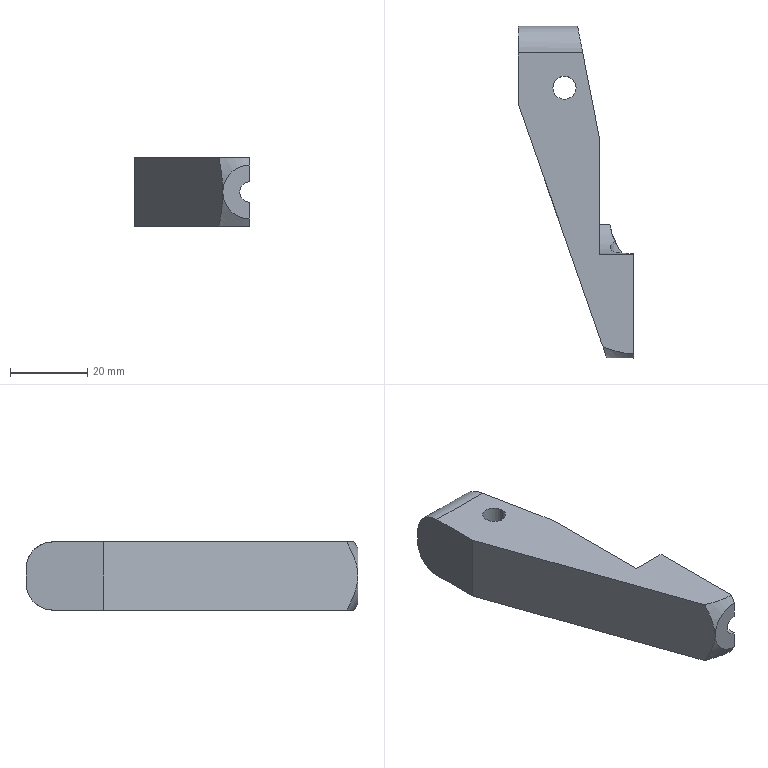Part | SolidWorks | features ICE 6, Extrusion 1, Fillet 1, RevCut 1 | 1 solid | 25 faces | box 30 x 86 x 17.7 mm | volume 18921 mm3 | plane 11 | cylinder 8 | spline 2 | torus 2 | cone 2 | commonest cylinder face diameters 6 x2 8 x2 14 x2 5.3 x1 12.388 x1
STEP:
#1=CARTESIAN_POINT('',(16.36,-5.,4.85));
#2=VERTEX_POINT('',#1);
#3=CARTESIAN_POINT('',(16.36,-5.,12.85));
#4=VERTEX_POINT('',#3);
#5=CARTESIAN_POINT('',(16.36,-5.,4.85));
#6=CARTESIAN_POINT('',(17.933,-13.,4.85));
#7=CARTESIAN_POINT('',(17.933,-13.,12.85));
#8=CARTESIAN_POINT('',(16.36,-5.,12.85));
#9=(BOUNDED_CURVE()B_SPLINE_CURVE(3,(#5,#6,#7,#8),.UNSPECIFIED.,.F.,.F.)B_SPLINE_CURVE_WITH_KNOTS((4,4),(1.571,4.712),.UNSPECIFIED.)CURVE()GEOMETRIC_REPRESENTATION_ITEM()RATIONAL_B_SPLINE_CURVE((1.,0.3333,0.3333,1.))REPRESENTATION_ITEM(''));
#10=EDGE_CURVE('',#2,#4,#9,.T.);
#11=ORIENTED_EDGE('',*,*,#10,.F.);
#12=CARTESIAN_POINT('',(6.,-5.,4.85));
#13=VERTEX_POINT('',#12);
#14=CARTESIAN_POINT('',(54.,-5.,4.85));
#15=DIRECTION('',(-1.,0.,0.));
#16=VECTOR('',#15,1000.);
#17=LINE('',#14,#16);
#18=EDGE_CURVE('',#2,#13,#17,.T.);
#19=ORIENTED_EDGE('',*,*,#18,.T.);
#20=CARTESIAN_POINT('',(6.,-5.,12.85));
#21=VERTEX_POINT('',#20);
#22=CARTESIAN_POINT('',(6.,-5.,8.85));
#23=DIRECTION('',(-1.,0.,0.));
#24=DIRECTION('',(0.,0.,1.));
#25=AXIS2_PLACEMENT_3D('',#22,#23,#24);
#26=CIRCLE('',#25,4.);
#27=EDGE_CURVE('',#13,#21,#26,.T.);
#28=ORIENTED_EDGE('',*,*,#27,.T.);
#29=CARTESIAN_POINT('',(54.,-5.,12.85));
#30=DIRECTION('',(-1.,0.,0.));
#31=VECTOR('',#30,1000.);
#32=LINE('',#29,#31);
#33=EDGE_CURVE('',#4,#21,#32,.T.);
#34=ORIENTED_EDGE('',*,*,#33,.F.);
#35=EDGE_LOOP('',(#11,#19,#28,#34));
#36=FACE_OUTER_BOUND('',#35,.T.);
#37=CARTESIAN_POINT('',(54.,-5.,8.85));
#38=DIRECTION('',(-1.,0.,0.));
#39=DIRECTION('',(0.,0.,1.));
#40=AXIS2_PLACEMENT_3D('',#37,#38,#39);
#41=CYLINDRICAL_SURFACE('',#40,4.);
#42=ADVANCED_FACE('',(#36),#41,.F.);
#43=CARTESIAN_POINT('',(9.,-16.,17.7));
#44=VERTEX_POINT('',#43);
#45=CARTESIAN_POINT('',(15.,-16.,17.7));
#46=VERTEX_POINT('',#45);
#47=CARTESIAN_POINT('',(12.,-16.,17.7));
#48=DIRECTION('',(0.,0.,1.));
#49=DIRECTION('',(1.,0.,0.));
#50=AXIS2_PLACEMENT_3D('',#47,#48,#49);
#51=CIRCLE('',#50,3.);
#52=EDGE_CURVE('',#44,#46,#51,.T.);
#53=ORIENTED_EDGE('',*,*,#52,.T.);
#54=CARTESIAN_POINT('',(15.,-16.,0.));
#55=VERTEX_POINT('',#54);
#56=CARTESIAN_POINT('',(15.,-16.,17.7));
#57=DIRECTION('',(0.,0.,-1.));
#58=VECTOR('',#57,1000.);
#59=LINE('',#56,#58);
#60=EDGE_CURVE('',#46,#55,#59,.T.);
#61=ORIENTED_EDGE('',*,*,#60,.T.);
#62=CARTESIAN_POINT('',(9.,-16.,0.));
#63=VERTEX_POINT('',#62);
#64=CARTESIAN_POINT('',(12.,-16.,0.));
#65=DIRECTION('',(0.,0.,1.));
#66=DIRECTION('',(1.,0.,0.));
#67=AXIS2_PLACEMENT_3D('',#64,#65,#66);
#68=CIRCLE('',#67,3.);
#69=EDGE_CURVE('',#63,#55,#68,.T.);
#70=ORIENTED_EDGE('',*,*,#69,.F.);
#71=CARTESIAN_POINT('',(9.,-16.,17.7));
#72=DIRECTION('',(0.,0.,-1.));
#73=VECTOR('',#72,1000.);
#74=LINE('',#71,#73);
#75=EDGE_CURVE('',#44,#63,#74,.T.);
#76=ORIENTED_EDGE('',*,*,#75,.F.);
#77=EDGE_LOOP('',(#53,#61,#70,#76));
#78=FACE_OUTER_BOUND('',#77,.T.);
#79=CARTESIAN_POINT('',(12.,-16.,17.7));
#80=DIRECTION('',(0.,0.,-1.));
#81=DIRECTION('',(-1.,0.,0.));
#82=AXIS2_PLACEMENT_3D('',#79,#80,#81);
#83=CYLINDRICAL_SURFACE('',#82,3.);
#84=ADVANCED_FACE('',(#78),#83,.F.);
#85=CARTESIAN_POINT('',(30.,-59.152,17.7));
#86=VERTEX_POINT('',#85);
#87=CARTESIAN_POINT('',(30.,-84.932,17.7));
#88=VERTEX_POINT('',#87);
#89=CARTESIAN_POINT('',(30.,-86.,17.7));
#90=DIRECTION('',(0.,-1.,0.));
#91=VECTOR('',#90,1000.);
#92=LINE('',#89,#91);
#93=EDGE_CURVE('',#86,#88,#92,.T.);
#94=ORIENTED_EDGE('',*,*,#93,.F.);
#95=CARTESIAN_POINT('',(21.,-59.152,17.7));
#96=VERTEX_POINT('',#95);
#97=CARTESIAN_POINT('',(58.282,-59.152,17.7));
#98=DIRECTION('',(-1.,0.,0.));
#99=VECTOR('',#98,1000.);
#100=LINE('',#97,#99);
#101=EDGE_CURVE('',#86,#96,#100,.T.);
#102=ORIENTED_EDGE('',*,*,#101,.T.);
#103=CARTESIAN_POINT('',(21.,-28.6,17.7));
#104=VERTEX_POINT('',#103);
#105=CARTESIAN_POINT('',(21.,-51.504,17.7));
#106=DIRECTION('',(0.,1.,0.));
#107=VECTOR('',#106,1000.);
#108=LINE('',#105,#107);
#109=EDGE_CURVE('',#96,#104,#108,.T.);
#110=ORIENTED_EDGE('',*,*,#109,.T.);
#111=CARTESIAN_POINT('',(16.753,-7.,17.7));
#112=VERTEX_POINT('',#111);
#113=CARTESIAN_POINT('',(21.,-28.6,17.7));
#114=DIRECTION('',(-0.1929,0.9812,0.));
#115=VECTOR('',#114,1000.);
#116=LINE('',#113,#115);
#117=EDGE_CURVE('',#104,#112,#116,.T.);
#118=ORIENTED_EDGE('',*,*,#117,.T.);
#119=CARTESIAN_POINT('',(0.,-7.,17.7));
#120=VERTEX_POINT('',#119);
#121=CARTESIAN_POINT('',(0.,-7.,17.7));
#122=DIRECTION('',(-1.,0.,0.));
#123=VECTOR('',#122,1000.);
#124=LINE('',#121,#123);
#125=EDGE_CURVE('',#112,#120,#124,.T.);
#126=ORIENTED_EDGE('',*,*,#125,.T.);
#127=CARTESIAN_POINT('',(0.,-20.136,17.7));
#128=VERTEX_POINT('',#127);
#129=CARTESIAN_POINT('',(0.,-20.136,17.7));
#130=DIRECTION('',(0.,-1.,0.));
#131=VECTOR('',#130,1000.);
#132=LINE('',#129,#131);
#133=EDGE_CURVE('',#120,#128,#132,.T.);
#134=ORIENTED_EDGE('',*,*,#133,.T.);
#135=CARTESIAN_POINT('',(21.049,-80.412,17.7));
#136=VERTEX_POINT('',#135);
#137=CARTESIAN_POINT('',(21.049,-80.412,17.7));
#138=DIRECTION('',(0.3297,-0.9441,0.));
#139=VECTOR('',#138,1000.);
#140=LINE('',#137,#139);
#141=EDGE_CURVE('',#128,#136,#140,.T.);
#142=ORIENTED_EDGE('',*,*,#141,.T.);
#143=CARTESIAN_POINT('',(21.669,-82.189,17.7));
#144=VERTEX_POINT('',#143);
#145=CARTESIAN_POINT('',(21.049,-80.412,17.7));
#146=CARTESIAN_POINT('',(21.259,-81.015,17.7));
#147=CARTESIAN_POINT('',(21.467,-81.609,17.7));
#148=CARTESIAN_POINT('',(21.669,-82.189,17.7));
#149=B_SPLINE_CURVE_WITH_KNOTS('',3,(#145,#146,#147,#148),.UNSPECIFIED.,.F.,.F.,(4,4),(0.75,1.),.UNSPECIFIED.);
#150=EDGE_CURVE('',#136,#144,#149,.T.);
#151=ORIENTED_EDGE('',*,*,#150,.T.);
#152=CARTESIAN_POINT('',(22.007,-83.156,17.7));
#153=VERTEX_POINT('',#152);
#154=CARTESIAN_POINT('',(21.669,-82.189,17.7));
#155=CARTESIAN_POINT('',(21.784,-82.517,17.7));
#156=CARTESIAN_POINT('',(21.897,-82.841,17.7));
#157=CARTESIAN_POINT('',(22.007,-83.156,17.7));
#158=B_SPLINE_CURVE_WITH_KNOTS('',3,(#154,#155,#156,#157),.UNSPECIFIED.,.F.,.F.,(4,4),(0.5,0.6415),.UNSPECIFIED.);
#159=EDGE_CURVE('',#144,#153,#158,.T.);
#160=ORIENTED_EDGE('',*,*,#159,.T.);
#161=CARTESIAN_POINT('',(22.007,-83.156,17.7));
#162=CARTESIAN_POINT('',(23.287,-83.652,17.7));
#163=CARTESIAN_POINT('',(24.588,-84.094,17.7));
#164=CARTESIAN_POINT('',(26.602,-84.58,17.7));
#165=CARTESIAN_POINT('',(27.28,-84.71,17.7));
#166=CARTESIAN_POINT('',(28.637,-84.886,17.7));
#167=CARTESIAN_POINT('',(29.317,-84.932,17.7));
#168=CARTESIAN_POINT('',(30.,-84.932,17.7));
#169=B_SPLINE_CURVE_WITH_KNOTS('',3,(#161,#162,#163,#164,#165,#166,#167,#168),.UNSPECIFIED.,.F.,.F.,(4,2,2,4),(0.1132,0.1173,0.1194,0.1214),.UNSPECIFIED.);
#170=EDGE_CURVE('',#153,#88,#169,.T.);
#171=ORIENTED_EDGE('',*,*,#170,.T.);
#172=EDGE_LOOP('',(#94,#102,#110,#118,#126,#134,#142,#151,#160,#171));
#173=FACE_OUTER_BOUND('',#172,.T.);
#174=ORIENTED_EDGE('',*,*,#52,.F.);
#175=CARTESIAN_POINT('',(12.,-16.,17.7));
#176=DIRECTION('',(0.,0.,1.));
#177=DIRECTION('',(1.,0.,0.));
#178=AXIS2_PLACEMENT_3D('',#175,#176,#177);
#179=CIRCLE('',#178,3.);
#180=EDGE_CURVE('',#46,#44,#179,.T.);
#181=ORIENTED_EDGE('',*,*,#180,.F.);
#182=EDGE_LOOP('',(#174,#181));
#183=FACE_BOUND('',#182,.T.);
#184=CARTESIAN_POINT('',(25.162,-51.504,17.7));
#185=DIRECTION('',(0.,0.,1.));
#186=DIRECTION('',(1.,0.,0.));
#187=AXIS2_PLACEMENT_3D('',#184,#185,#186);
#188=PLANE('',#187);
#189=ADVANCED_FACE('',(#173,#183),#188,.T.);
#190=ORIENTED_EDGE('',*,*,#69,.T.);
#191=CARTESIAN_POINT('',(12.,-16.,0.));
#192=DIRECTION('',(0.,0.,1.));
#193=DIRECTION('',(1.,0.,0.));
#194=AXIS2_PLACEMENT_3D('',#191,#192,#193);
#195=CIRCLE('',#194,3.);
#196=EDGE_CURVE('',#55,#63,#195,.T.);
#197=ORIENTED_EDGE('',*,*,#196,.T.);
#198=EDGE_LOOP('',(#190,#197));
#199=FACE_BOUND('',#198,.T.);
#200=CARTESIAN_POINT('',(30.,-60.226,0.));
#201=VERTEX_POINT('',#200);
#202=CARTESIAN_POINT('',(23.784,-51.504,0.));
#203=VERTEX_POINT('',#202);
#204=CARTESIAN_POINT('',(30.,-60.226,0.));
#205=CARTESIAN_POINT('',(27.027,-60.226,0.));
#206=CARTESIAN_POINT('',(24.641,-56.878,0.));
#207=CARTESIAN_POINT('',(23.784,-51.504,0.));
#208=(BOUNDED_CURVE()B_SPLINE_CURVE(3,(#204,#205,#206,#207),.UNSPECIFIED.,.F.,.F.)B_SPLINE_CURVE_WITH_KNOTS((4,4),(3.142,4.42),.UNSPECIFIED.)CURVE()GEOMETRIC_REPRESENTATION_ITEM()RATIONAL_B_SPLINE_CURVE((1.,0.8684,0.8684,1.))REPRESENTATION_ITEM(''));
#209=EDGE_CURVE('',#201,#203,#208,.T.);
#210=ORIENTED_EDGE('',*,*,#209,.F.);
#211=CARTESIAN_POINT('',(30.,-84.932,0.));
#212=VERTEX_POINT('',#211);
#213=CARTESIAN_POINT('',(30.,-51.504,0.));
#214=DIRECTION('',(0.,-1.,0.));
#215=VECTOR('',#214,1000.);
#216=LINE('',#213,#215);
#217=EDGE_CURVE('',#201,#212,#216,.T.);
#218=ORIENTED_EDGE('',*,*,#217,.T.);
#219=CARTESIAN_POINT('',(22.007,-83.156,0.));
#220=VERTEX_POINT('',#219);
#221=CARTESIAN_POINT('',(22.007,-83.156,0.));
#222=CARTESIAN_POINT('',(23.287,-83.652,0.));
#223=CARTESIAN_POINT('',(24.588,-84.094,0.));
#224=CARTESIAN_POINT('',(26.602,-84.58,0.));
#225=CARTESIAN_POINT('',(27.28,-84.71,0.));
#226=CARTESIAN_POINT('',(28.637,-84.886,0.));
#227=CARTESIAN_POINT('',(29.317,-84.932,0.));
#228=CARTESIAN_POINT('',(30.,-84.932,0.));
#229=B_SPLINE_CURVE_WITH_KNOTS('',3,(#221,#222,#223,#224,#225,#226,#227,#228),.UNSPECIFIED.,.F.,.F.,(4,2,2,4),(0.1132,0.1173,0.1194,0.1214),.UNSPECIFIED.);
#230=EDGE_CURVE('',#220,#212,#229,.T.);
#231=ORIENTED_EDGE('',*,*,#230,.F.);
#232=CARTESIAN_POINT('',(21.669,-82.189,0.));
#233=VERTEX_POINT('',#232);
#234=CARTESIAN_POINT('',(21.669,-82.189,0.));
#235=CARTESIAN_POINT('',(21.784,-82.517,0.));
#236=CARTESIAN_POINT('',(21.897,-82.841,0.));
#237=CARTESIAN_POINT('',(22.007,-83.156,0.));
#238=B_SPLINE_CURVE_WITH_KNOTS('',3,(#234,#235,#236,#237),.UNSPECIFIED.,.F.,.F.,(4,4),(0.5,0.6415),.UNSPECIFIED.);
#239=EDGE_CURVE('',#233,#220,#238,.T.);
#240=ORIENTED_EDGE('',*,*,#239,.F.);
#241=CARTESIAN_POINT('',(21.049,-80.412,0.));
#242=VERTEX_POINT('',#241);
#243=CARTESIAN_POINT('',(21.049,-80.412,0.));
#244=CARTESIAN_POINT('',(21.259,-81.015,0.));
#245=CARTESIAN_POINT('',(21.467,-81.609,0.));
#246=CARTESIAN_POINT('',(21.669,-82.189,0.));
#247=B_SPLINE_CURVE_WITH_KNOTS('',3,(#243,#244,#245,#246),.UNSPECIFIED.,.F.,.F.,(4,4),(0.75,1.),.UNSPECIFIED.);
#248=EDGE_CURVE('',#242,#233,#247,.T.);
#249=ORIENTED_EDGE('',*,*,#248,.F.);
#250=CARTESIAN_POINT('',(0.,-20.136,0.));
#251=VERTEX_POINT('',#250);
#252=CARTESIAN_POINT('',(21.049,-80.412,0.));
#253=DIRECTION('',(0.3297,-0.9441,0.));
#254=VECTOR('',#253,1000.);
#255=LINE('',#252,#254);
#256=EDGE_CURVE('',#251,#242,#255,.T.);
#257=ORIENTED_EDGE('',*,*,#256,.F.);
#258=CARTESIAN_POINT('',(0.,-7.,0.));
#259=VERTEX_POINT('',#258);
#260=CARTESIAN_POINT('',(0.,-20.136,0.));
#261=DIRECTION('',(0.,-1.,0.));
#262=VECTOR('',#261,1000.);
#263=LINE('',#260,#262);
#264=EDGE_CURVE('',#259,#251,#263,.T.);
#265=ORIENTED_EDGE('',*,*,#264,.F.);
#266=CARTESIAN_POINT('',(16.753,-7.,0.));
#267=VERTEX_POINT('',#266);
#268=CARTESIAN_POINT('',(25.162,-7.,0.));
#269=DIRECTION('',(1.,0.,0.));
#270=VECTOR('',#269,1000.);
#271=LINE('',#268,#270);
#272=EDGE_CURVE('',#259,#267,#271,.T.);
#273=ORIENTED_EDGE('',*,*,#272,.T.);
#274=CARTESIAN_POINT('',(21.,-28.6,0.));
#275=VERTEX_POINT('',#274);
#276=CARTESIAN_POINT('',(21.,-28.6,0.));
#277=DIRECTION('',(-0.1929,0.9812,0.));
#278=VECTOR('',#277,1000.);
#279=LINE('',#276,#278);
#280=EDGE_CURVE('',#275,#267,#279,.T.);
#281=ORIENTED_EDGE('',*,*,#280,.F.);
#282=CARTESIAN_POINT('',(21.,-51.504,0.));
#283=VERTEX_POINT('',#282);
#284=CARTESIAN_POINT('',(21.,-51.504,0.));
#285=DIRECTION('',(0.,1.,0.));
#286=VECTOR('',#285,1000.);
#287=LINE('',#284,#286);
#288=EDGE_CURVE('',#283,#275,#287,.T.);
#289=ORIENTED_EDGE('',*,*,#288,.F.);
#290=CARTESIAN_POINT('',(39.,-51.504,0.));
#291=DIRECTION('',(-1.,0.,0.));
#292=VECTOR('',#291,1000.);
#293=LINE('',#290,#292);
#294=EDGE_CURVE('',#203,#283,#293,.T.);
#295=ORIENTED_EDGE('',*,*,#294,.F.);
#296=EDGE_LOOP('',(#210,#218,#231,#240,#249,#257,#265,#273,#281,#289,#295));
#297=FACE_OUTER_BOUND('',#296,.T.);
#298=CARTESIAN_POINT('',(25.162,-51.504,0.));
#299=DIRECTION('',(0.,0.,1.));
#300=DIRECTION('',(1.,0.,0.));
#301=AXIS2_PLACEMENT_3D('',#298,#299,#300);
#302=PLANE('',#301);
#303=ADVANCED_FACE('',(#199,#297),#302,.F.);
#304=CARTESIAN_POINT('',(23.,-86.,8.85));
#305=VERTEX_POINT('',#304);
#306=CARTESIAN_POINT('',(22.007,-83.156,17.7));
#307=CARTESIAN_POINT('',(22.128,-83.502,17.003));
#308=CARTESIAN_POINT('',(22.245,-83.838,16.301));
#309=CARTESIAN_POINT('',(22.468,-84.477,14.881));
#310=CARTESIAN_POINT('',(22.574,-84.78,14.163));
#311=CARTESIAN_POINT('',(22.763,-85.321,12.697));
#312=CARTESIAN_POINT('',(22.846,-85.56,11.945));
#313=CARTESIAN_POINT('',(22.965,-85.9,10.42));
#314=CARTESIAN_POINT('',(23.,-86.,9.644));
#315=CARTESIAN_POINT('',(23.,-86.,8.85));
#316=B_SPLINE_CURVE_WITH_KNOTS('',3,(#306,#307,#308,#309,#310,#311,#312,#313,#314,#315),.UNSPECIFIED.,.F.,.F.,(4,2,2,2,4),(0.000000225,0.002359,0.004717,0.007076,0.009434),.UNSPECIFIED.);
#317=EDGE_CURVE('',#153,#305,#316,.T.);
#318=ORIENTED_EDGE('',*,*,#317,.F.);
#319=ORIENTED_EDGE('',*,*,#159,.F.);
#320=ORIENTED_EDGE('',*,*,#150,.F.);
#321=ORIENTED_EDGE('',*,*,#141,.F.);
#322=CARTESIAN_POINT('',(0.,-20.136,17.7));
#323=DIRECTION('',(0.,0.,-1.));
#324=VECTOR('',#323,1000.);
#325=LINE('',#322,#324);
#326=EDGE_CURVE('',#128,#251,#325,.T.);
#327=ORIENTED_EDGE('',*,*,#326,.T.);
#328=ORIENTED_EDGE('',*,*,#256,.T.);
#329=ORIENTED_EDGE('',*,*,#248,.T.);
#330=ORIENTED_EDGE('',*,*,#239,.T.);
#331=CARTESIAN_POINT('',(23.,-86.,8.85));
#332=CARTESIAN_POINT('',(23.,-86.,8.056));
#333=CARTESIAN_POINT('',(22.965,-85.9,7.279));
#334=CARTESIAN_POINT('',(22.846,-85.56,5.755));
#335=CARTESIAN_POINT('',(22.763,-85.321,5.003));
#336=CARTESIAN_POINT('',(22.574,-84.78,3.537));
#337=CARTESIAN_POINT('',(22.468,-84.477,2.819));
#338=CARTESIAN_POINT('',(22.245,-83.838,1.399));
#339=CARTESIAN_POINT('',(22.128,-83.502,0.6974));
#340=CARTESIAN_POINT('',(22.007,-83.156,0.));
#341=B_SPLINE_CURVE_WITH_KNOTS('',3,(#331,#332,#333,#334,#335,#336,#337,#338,#339,#340),.UNSPECIFIED.,.F.,.F.,(4,2,2,2,4),(0.009434,0.01179,0.01415,0.01651,0.01886),.UNSPECIFIED.);
#342=EDGE_CURVE('',#305,#220,#341,.T.);
#343=ORIENTED_EDGE('',*,*,#342,.F.);
#344=EDGE_LOOP('',(#318,#319,#320,#321,#327,#328,#329,#330,#343));
#345=FACE_OUTER_BOUND('',#344,.T.);
#346=CARTESIAN_POINT('',(22.932,-85.807,17.7));
#347=DIRECTION('',(0.9441,0.3297,0.));
#348=DIRECTION('',(-0.3297,0.9441,0.));
#349=AXIS2_PLACEMENT_3D('',#346,#347,#348);
#350=PLANE('',#349);
#351=ADVANCED_FACE('',(#345),#350,.F.);
#352=CARTESIAN_POINT('',(30.,-86.,1.85));
#353=VERTEX_POINT('',#352);
#354=CARTESIAN_POINT('',(30.,-86.,8.85));
#355=DIRECTION('',(0.,-1.,0.));
#356=DIRECTION('',(0.,0.,-1.));
#357=AXIS2_PLACEMENT_3D('',#354,#355,#356);
#358=CIRCLE('',#357,7.);
#359=EDGE_CURVE('',#305,#353,#358,.T.);
#360=ORIENTED_EDGE('',*,*,#359,.T.);
#361=CARTESIAN_POINT('',(30.,-86.,6.2));
#362=VERTEX_POINT('',#361);
#363=CARTESIAN_POINT('',(30.,-86.,-26.3));
#364=DIRECTION('',(0.,0.,1.));
#365=VECTOR('',#364,1000.);
#366=LINE('',#363,#365);
#367=EDGE_CURVE('',#353,#362,#366,.T.);
#368=ORIENTED_EDGE('',*,*,#367,.T.);
#369=CARTESIAN_POINT('',(30.,-86.,11.5));
#370=VERTEX_POINT('',#369);
#371=CARTESIAN_POINT('',(30.,-86.,8.85));
#372=DIRECTION('',(0.,-1.,0.));
#373=DIRECTION('',(0.,0.,-1.));
#374=AXIS2_PLACEMENT_3D('',#371,#372,#373);
#375=CIRCLE('',#374,2.65);
#376=EDGE_CURVE('',#370,#362,#375,.T.);
#377=ORIENTED_EDGE('',*,*,#376,.F.);
#378=CARTESIAN_POINT('',(30.,-86.,15.85));
#379=VERTEX_POINT('',#378);
#380=CARTESIAN_POINT('',(30.,-86.,-26.3));
#381=DIRECTION('',(0.,0.,1.));
#382=VECTOR('',#381,1000.);
#383=LINE('',#380,#382);
#384=EDGE_CURVE('',#370,#379,#383,.T.);
#385=ORIENTED_EDGE('',*,*,#384,.T.);
#386=CARTESIAN_POINT('',(30.,-86.,8.85));
#387=DIRECTION('',(0.,-1.,0.));
#388=DIRECTION('',(0.,0.,-1.));
#389=AXIS2_PLACEMENT_3D('',#386,#387,#388);
#390=CIRCLE('',#389,7.);
#391=EDGE_CURVE('',#379,#305,#390,.T.);
#392=ORIENTED_EDGE('',*,*,#391,.T.);
#393=EDGE_LOOP('',(#360,#368,#377,#385,#392));
#394=FACE_OUTER_BOUND('',#393,.T.);
#395=CARTESIAN_POINT('',(37.,-86.,17.7));
#396=DIRECTION('',(0.,1.,0.));
#397=DIRECTION('',(0.,0.,1.));
#398=AXIS2_PLACEMENT_3D('',#395,#396,#397);
#399=PLANE('',#398);
#400=ADVANCED_FACE('',(#394),#399,.F.);
#401=CARTESIAN_POINT('',(30.,-75.,15.044));
#402=VERTEX_POINT('',#401);
#403=CARTESIAN_POINT('',(30.,-75.,2.656));
#404=VERTEX_POINT('',#403);
#405=CARTESIAN_POINT('',(30.,-75.,8.85));
#406=DIRECTION('',(0.,-1.,0.));
#407=DIRECTION('',(0.,0.,-1.));
#408=AXIS2_PLACEMENT_3D('',#405,#406,#407);
#409=CIRCLE('',#408,6.194);
#410=EDGE_CURVE('',#402,#404,#409,.T.);
#411=ORIENTED_EDGE('',*,*,#410,.T.);
#412=CARTESIAN_POINT('',(30.,-60.226,2.656));
#413=VERTEX_POINT('',#412);
#414=CARTESIAN_POINT('',(30.,-86.,2.656));
#415=DIRECTION('',(0.,1.,0.));
#416=VECTOR('',#415,1000.);
#417=LINE('',#414,#416);
#418=EDGE_CURVE('',#404,#413,#417,.T.);
#419=ORIENTED_EDGE('',*,*,#418,.T.);
#420=CARTESIAN_POINT('',(24.963,-55.701,5.246));
#421=VERTEX_POINT('',#420);
#422=CARTESIAN_POINT('',(24.963,-55.701,5.246));
#423=CARTESIAN_POINT('',(25.181,-56.209,4.94));
#424=CARTESIAN_POINT('',(25.433,-56.711,4.646));
#425=CARTESIAN_POINT('',(25.879,-57.448,4.221));
#426=CARTESIAN_POINT('',(26.04,-57.69,4.082));
#427=CARTESIAN_POINT('',(26.385,-58.158,3.815));
#428=CARTESIAN_POINT('',(26.57,-58.385,3.687));
#429=CARTESIAN_POINT('',(26.97,-58.818,3.443));
#430=CARTESIAN_POINT('',(27.185,-59.024,3.327));
#431=CARTESIAN_POINT('',(27.657,-59.41,3.11));
#432=CARTESIAN_POINT('',(27.908,-59.585,3.013));
#433=CARTESIAN_POINT('',(28.451,-59.884,2.846));
#434=CARTESIAN_POINT('',(28.745,-60.009,2.776));
#435=CARTESIAN_POINT('',(29.355,-60.18,2.682));
#436=CARTESIAN_POINT('',(29.68,-60.226,2.656));
#437=CARTESIAN_POINT('',(30.,-60.226,2.656));
#438=B_SPLINE_CURVE_WITH_KNOTS('',3,(#422,#423,#424,#425,#426,#427,#428,#429,#430,#431,#432,#433,#434,#435,#436,#437),.UNSPECIFIED.,.F.,.F.,(4,2,2,2,2,2,2,4),(-0.002276,-0.0003627,0.0005938,0.00155,0.002507,0.003463,0.00442,0.005376),.UNSPECIFIED.);
#439=EDGE_CURVE('',#421,#413,#438,.T.);
#440=ORIENTED_EDGE('',*,*,#439,.F.);
#441=CARTESIAN_POINT('',(30.,-58.989,15.044));
#442=VERTEX_POINT('',#441);
#443=CARTESIAN_POINT('',(24.963,-55.701,5.246));
#444=CARTESIAN_POINT('',(24.652,-55.963,5.68));
#445=CARTESIAN_POINT('',(24.403,-56.224,6.144));
#446=CARTESIAN_POINT('',(24.119,-56.608,6.887));
#447=CARTESIAN_POINT('',(24.039,-56.735,7.144));
#448=CARTESIAN_POINT('',(23.914,-56.982,7.668));
#449=CARTESIAN_POINT('',(23.868,-57.101,7.935));
#450=CARTESIAN_POINT('',(23.811,-57.332,8.476));
#451=CARTESIAN_POINT('',(23.801,-57.443,8.752));
#452=CARTESIAN_POINT('',(23.816,-57.654,9.305));
#453=CARTESIAN_POINT('',(23.843,-57.754,9.58));
#454=CARTESIAN_POINT('',(23.933,-57.94,10.129));
#455=CARTESIAN_POINT('',(23.997,-58.027,10.402));
#456=CARTESIAN_POINT('',(24.164,-58.189,10.946));
#457=CARTESIAN_POINT('',(24.268,-58.264,11.215));
#458=CARTESIAN_POINT('',(24.51,-58.4,11.732));
#459=CARTESIAN_POINT('',(24.649,-58.461,11.983));
#460=CARTESIAN_POINT('',(24.963,-58.571,12.467));
#461=CARTESIAN_POINT('',(25.14,-58.62,12.702));
#462=CARTESIAN_POINT('',(25.717,-58.751,13.363));
#463=CARTESIAN_POINT('',(26.158,-58.814,13.744));
#464=CARTESIAN_POINT('',(27.155,-58.91,14.384));
#465=CARTESIAN_POINT('',(27.69,-58.94,14.627));
#466=CARTESIAN_POINT('',(28.539,-58.97,14.877));
#467=CARTESIAN_POINT('',(28.831,-58.978,14.94));
#468=CARTESIAN_POINT('',(29.414,-58.987,15.023));
#469=CARTESIAN_POINT('',(29.706,-58.989,15.044));
#470=CARTESIAN_POINT('',(30.,-58.989,15.044));
#471=B_SPLINE_CURVE_WITH_KNOTS('',3,(#443,#444,#445,#446,#447,#448,#449,#450,#451,#452,#453,#454,#455,#456,#457,#458,#459,#460,#461,#462,#463,#464,#465,#466,#467,#468,#469,#470),.UNSPECIFIED.,.F.,.F.,(4,2,2,2,2,2,2,2,2,2,2,2,2,4),(0.03628,0.03804,0.03892,0.0398,0.04068,0.04156,0.04244,0.04332,0.0442,0.04508,0.04684,0.0486,0.04948,0.05036),.UNSPECIFIED.);
#472=EDGE_CURVE('',#421,#442,#471,.T.);
#473=ORIENTED_EDGE('',*,*,#472,.T.);
#474=CARTESIAN_POINT('',(30.,-86.,15.044));
#475=DIRECTION('',(0.,-1.,0.));
#476=VECTOR('',#475,1000.);
#477=LINE('',#474,#476);
#478=EDGE_CURVE('',#442,#402,#477,.T.);
#479=ORIENTED_EDGE('',*,*,#478,.T.);
#480=EDGE_LOOP('',(#411,#419,#440,#473,#479));
#481=FACE_OUTER_BOUND('',#480,.T.);
#482=CARTESIAN_POINT('',(30.,-86.,8.85));
#483=DIRECTION('',(0.,-1.,0.));
#484=DIRECTION('',(0.,0.,-1.));
#485=AXIS2_PLACEMENT_3D('',#482,#483,#484);
#486=CYLINDRICAL_SURFACE('',#485,6.194);
#487=ADVANCED_FACE('',(#481),#486,.F.);
#488=ORIENTED_EDGE('',*,*,#101,.F.);
#489=CARTESIAN_POINT('',(30.,-59.152,17.7));
#490=CARTESIAN_POINT('',(30.,-59.134,16.346));
#491=CARTESIAN_POINT('',(30.,-58.989,15.044));
#492=B_SPLINE_CURVE_WITH_KNOTS('',2,(#489,#490,#491),.UNSPECIFIED.,.F.,.F.,(3,3),(0.,0.1306),.UNSPECIFIED.);
#493=EDGE_CURVE('',#86,#442,#492,.T.);
#494=ORIENTED_EDGE('',*,*,#493,.T.);
#495=ORIENTED_EDGE('',*,*,#472,.F.);
#496=CARTESIAN_POINT('',(23.784,-51.504,0.));
#497=CARTESIAN_POINT('',(23.913,-52.315,0.7934));
#498=CARTESIAN_POINT('',(24.083,-53.075,1.625));
#499=CARTESIAN_POINT('',(24.484,-54.481,3.377));
#500=CARTESIAN_POINT('',(24.715,-55.125,4.292));
#501=CARTESIAN_POINT('',(24.963,-55.701,5.246));
#502=B_SPLINE_CURVE_WITH_KNOTS('',3,(#496,#497,#498,#499,#500,#501),.UNSPECIFIED.,.F.,.F.,(4,2,4),(0.,0.003417,0.006834),.UNSPECIFIED.);
#503=EDGE_CURVE('',#203,#421,#502,.T.);
#504=ORIENTED_EDGE('',*,*,#503,.F.);
#505=ORIENTED_EDGE('',*,*,#294,.T.);
#506=CARTESIAN_POINT('',(21.,-51.504,0.));
#507=CARTESIAN_POINT('',(21.,-59.009,7.335));
#508=CARTESIAN_POINT('',(21.,-59.152,17.7));
#509=B_SPLINE_CURVE_WITH_KNOTS('',2,(#506,#507,#508),.UNSPECIFIED.,.F.,.F.,(3,3),(0.,1.),.UNSPECIFIED.);
#510=EDGE_CURVE('',#283,#96,#509,.T.);
#511=ORIENTED_EDGE('',*,*,#510,.T.);
#512=EDGE_LOOP('',(#488,#494,#495,#504,#505,#511));
#513=FACE_OUTER_BOUND('',#512,.T.);
#514=CARTESIAN_POINT('',(30.,-51.504,0.));
#515=CARTESIAN_POINT('',(21.,-51.504,0.));
#516=CARTESIAN_POINT('',(30.,-59.009,7.335));
#517=CARTESIAN_POINT('',(21.,-59.009,7.335));
#518=CARTESIAN_POINT('',(30.,-59.152,17.7));
#519=CARTESIAN_POINT('',(21.,-59.152,17.7));
#520=B_SPLINE_SURFACE_WITH_KNOTS('',2,1,((#514,#515),(#516,#517),(#518,#519)),.UNSPECIFIED.,.F.,.F.,.F.,(3,3),(2,2),(0.,1.),(0.,1.),.UNSPECIFIED.);
#521=ADVANCED_FACE('',(#513),#520,.F.);
#522=ORIENTED_EDGE('',*,*,#288,.T.);
#523=CARTESIAN_POINT('',(21.,-28.6,17.7));
#524=DIRECTION('',(0.,0.,-1.));
#525=VECTOR('',#524,1000.);
#526=LINE('',#523,#525);
#527=EDGE_CURVE('',#104,#275,#526,.T.);
#528=ORIENTED_EDGE('',*,*,#527,.F.);
#529=ORIENTED_EDGE('',*,*,#109,.F.);
#530=ORIENTED_EDGE('',*,*,#510,.F.);
#531=EDGE_LOOP('',(#522,#528,#529,#530));
#532=FACE_OUTER_BOUND('',#531,.T.);
#533=CARTESIAN_POINT('',(21.,-51.504,17.7));
#534=DIRECTION('',(-1.,0.,0.));
#535=DIRECTION('',(0.,0.,1.));
#536=AXIS2_PLACEMENT_3D('',#533,#534,#535);
#537=PLANE('',#536);
#538=ADVANCED_FACE('',(#532),#537,.F.);
#539=CARTESIAN_POINT('',(16.36,-5.,12.85));
#540=CARTESIAN_POINT('',(14.787,3.,12.85));
#541=CARTESIAN_POINT('',(14.787,3.,4.85));
#542=CARTESIAN_POINT('',(16.36,-5.,4.85));
#543=(BOUNDED_CURVE()B_SPLINE_CURVE(3,(#539,#540,#541,#542),.UNSPECIFIED.,.F.,.F.)B_SPLINE_CURVE_WITH_KNOTS((4,4),(4.712,7.854),.UNSPECIFIED.)CURVE()GEOMETRIC_REPRESENTATION_ITEM()RATIONAL_B_SPLINE_CURVE((1.,0.3333,0.3333,1.))REPRESENTATION_ITEM(''));
#544=EDGE_CURVE('',#4,#2,#543,.T.);
#545=ORIENTED_EDGE('',*,*,#544,.T.);
#546=ORIENTED_EDGE('',*,*,#10,.T.);
#547=EDGE_LOOP('',(#545,#546));
#548=FACE_BOUND('',#547,.T.);
#549=ORIENTED_EDGE('',*,*,#280,.T.);
#550=CARTESIAN_POINT('',(15.376,0.,7.));
#551=VERTEX_POINT('',#550);
#552=CARTESIAN_POINT('',(16.753,-7.,0.));
#553=CARTESIAN_POINT('',(15.947,-2.899,0.));
#554=CARTESIAN_POINT('',(15.376,0.,2.899));
#555=CARTESIAN_POINT('',(15.376,0.,7.));
#556=(BOUNDED_CURVE()B_SPLINE_CURVE(3,(#552,#553,#554,#555),.UNSPECIFIED.,.F.,.F.)B_SPLINE_CURVE_WITH_KNOTS((4,4),(4.712,6.283),.UNSPECIFIED.)CURVE()GEOMETRIC_REPRESENTATION_ITEM()RATIONAL_B_SPLINE_CURVE((1.,0.8047,0.8047,1.))REPRESENTATION_ITEM(''));
#557=EDGE_CURVE('',#267,#551,#556,.T.);
#558=ORIENTED_EDGE('',*,*,#557,.T.);
#559=CARTESIAN_POINT('',(15.376,0.,10.7));
#560=VERTEX_POINT('',#559);
#561=CARTESIAN_POINT('',(15.376,0.,17.7));
#562=DIRECTION('',(0.,0.,-1.));
#563=VECTOR('',#562,1000.);
#564=LINE('',#561,#563);
#565=EDGE_CURVE('',#560,#551,#564,.T.);
#566=ORIENTED_EDGE('',*,*,#565,.F.);
#567=CARTESIAN_POINT('',(15.376,0.,10.7));
#568=CARTESIAN_POINT('',(15.376,0.,14.801));
#569=CARTESIAN_POINT('',(15.947,-2.899,17.7));
#570=CARTESIAN_POINT('',(16.753,-7.,17.7));
#571=(BOUNDED_CURVE()B_SPLINE_CURVE(3,(#567,#568,#569,#570),.UNSPECIFIED.,.F.,.F.)B_SPLINE_CURVE_WITH_KNOTS((4,4),(3.142,4.712),.UNSPECIFIED.)CURVE()GEOMETRIC_REPRESENTATION_ITEM()RATIONAL_B_SPLINE_CURVE((1.,0.8047,0.8047,1.))REPRESENTATION_ITEM(''));
#572=EDGE_CURVE('',#560,#112,#571,.T.);
#573=ORIENTED_EDGE('',*,*,#572,.T.);
#574=ORIENTED_EDGE('',*,*,#117,.F.);
#575=ORIENTED_EDGE('',*,*,#527,.T.);
#576=EDGE_LOOP('',(#549,#558,#566,#573,#574,#575));
#577=FACE_OUTER_BOUND('',#576,.T.);
#578=CARTESIAN_POINT('',(21.,-28.6,17.7));
#579=DIRECTION('',(-0.9812,-0.1929,0.));
#580=DIRECTION('',(0.1929,-0.9812,0.));
#581=AXIS2_PLACEMENT_3D('',#578,#579,#580);
#582=PLANE('',#581);
#583=ADVANCED_FACE('',(#548,#577),#582,.F.);
#584=ORIENTED_EDGE('',*,*,#565,.T.);
#585=CARTESIAN_POINT('',(0.,0.,7.));
#586=VERTEX_POINT('',#585);
#587=CARTESIAN_POINT('',(0.,0.,7.));
#588=DIRECTION('',(-1.,0.,0.));
#589=VECTOR('',#588,1000.);
#590=LINE('',#587,#589);
#591=EDGE_CURVE('',#551,#586,#590,.T.);
#592=ORIENTED_EDGE('',*,*,#591,.T.);
#593=CARTESIAN_POINT('',(0.,0.,10.7));
#594=VERTEX_POINT('',#593);
#595=CARTESIAN_POINT('',(0.,0.,17.7));
#596=DIRECTION('',(0.,0.,-1.));
#597=VECTOR('',#596,1000.);
#598=LINE('',#595,#597);
#599=EDGE_CURVE('',#594,#586,#598,.T.);
#600=ORIENTED_EDGE('',*,*,#599,.F.);
#601=CARTESIAN_POINT('',(15.376,0.,10.7));
#602=DIRECTION('',(1.,0.,0.));
#603=VECTOR('',#602,1000.);
#604=LINE('',#601,#603);
#605=EDGE_CURVE('',#594,#560,#604,.T.);
#606=ORIENTED_EDGE('',*,*,#605,.T.);
#607=EDGE_LOOP('',(#584,#592,#600,#606));
#608=FACE_OUTER_BOUND('',#607,.T.);
#609=CARTESIAN_POINT('',(0.,0.,17.7));
#610=DIRECTION('',(0.,-1.,0.));
#611=DIRECTION('',(0.,0.,-1.));
#612=AXIS2_PLACEMENT_3D('',#609,#610,#611);
#613=PLANE('',#612);
#614=ADVANCED_FACE('',(#608),#613,.F.);
#615=ORIENTED_EDGE('',*,*,#599,.T.);
#616=CARTESIAN_POINT('',(0.,-7.,7.));
#617=DIRECTION('',(-1.,0.,0.));
#618=DIRECTION('',(0.,0.,-1.));
#619=AXIS2_PLACEMENT_3D('',#616,#617,#618);
#620=CIRCLE('',#619,7.);
#621=EDGE_CURVE('',#586,#259,#620,.T.);
#622=ORIENTED_EDGE('',*,*,#621,.T.);
#623=ORIENTED_EDGE('',*,*,#264,.T.);
#624=ORIENTED_EDGE('',*,*,#326,.F.);
#625=ORIENTED_EDGE('',*,*,#133,.F.);
#626=CARTESIAN_POINT('',(0.,-7.,10.7));
#627=DIRECTION('',(-1.,0.,0.));
#628=DIRECTION('',(0.,0.,-1.));
#629=AXIS2_PLACEMENT_3D('',#626,#627,#628);
#630=CIRCLE('',#629,7.);
#631=EDGE_CURVE('',#120,#594,#630,.T.);
#632=ORIENTED_EDGE('',*,*,#631,.T.);
#633=EDGE_LOOP('',(#615,#622,#623,#624,#625,#632));
#634=FACE_OUTER_BOUND('',#633,.T.);
#635=CARTESIAN_POINT('',(0.,-20.136,17.7));
#636=DIRECTION('',(1.,0.,0.));
#637=DIRECTION('',(0.,0.,-1.));
#638=AXIS2_PLACEMENT_3D('',#635,#636,#637);
#639=PLANE('',#638);
#640=ADVANCED_FACE('',(#634),#639,.F.);
#641=ORIENTED_EDGE('',*,*,#60,.F.);
#642=ORIENTED_EDGE('',*,*,#180,.T.);
#643=ORIENTED_EDGE('',*,*,#75,.T.);
#644=ORIENTED_EDGE('',*,*,#196,.F.);
#645=EDGE_LOOP('',(#641,#642,#643,#644));
#646=FACE_OUTER_BOUND('',#645,.T.);
#647=CARTESIAN_POINT('',(12.,-16.,17.7));
#648=DIRECTION('',(0.,0.,-1.));
#649=DIRECTION('',(-1.,0.,0.));
#650=AXIS2_PLACEMENT_3D('',#647,#648,#649);
#651=CYLINDRICAL_SURFACE('',#650,3.);
#652=ADVANCED_FACE('',(#646),#651,.F.);
#653=CARTESIAN_POINT('',(30.,-81.75,11.5));
#654=VERTEX_POINT('',#653);
#655=CARTESIAN_POINT('',(30.,-81.75,6.2));
#656=VERTEX_POINT('',#655);
#657=CARTESIAN_POINT('',(30.,-81.75,8.85));
#658=DIRECTION('',(0.,-1.,0.));
#659=DIRECTION('',(0.,0.,-1.));
#660=AXIS2_PLACEMENT_3D('',#657,#658,#659);
#661=CIRCLE('',#660,2.65);
#662=EDGE_CURVE('',#654,#656,#661,.T.);
#663=ORIENTED_EDGE('',*,*,#662,.T.);
#664=CARTESIAN_POINT('',(30.,-80.104,5.336));
#665=VERTEX_POINT('',#664);
#666=CARTESIAN_POINT('',(30.,-81.75,4.2));
#667=DIRECTION('',(-1.,0.,0.));
#668=DIRECTION('',(0.,0.,1.));
#669=AXIS2_PLACEMENT_3D('',#666,#667,#668);
#670=CIRCLE('',#669,2.);
#671=EDGE_CURVE('',#656,#665,#670,.T.);
#672=ORIENTED_EDGE('',*,*,#671,.T.);
#673=CARTESIAN_POINT('',(30.,-80.104,12.364));
#674=VERTEX_POINT('',#673);
#675=CARTESIAN_POINT('',(30.,-80.104,8.85));
#676=DIRECTION('',(0.,-1.,0.));
#677=DIRECTION('',(0.,0.,-1.));
#678=AXIS2_PLACEMENT_3D('',#675,#676,#677);
#679=CIRCLE('',#678,3.514);
#680=EDGE_CURVE('',#674,#665,#679,.T.);
#681=ORIENTED_EDGE('',*,*,#680,.F.);
#682=CARTESIAN_POINT('',(30.,-81.75,13.5));
#683=DIRECTION('',(-1.,0.,0.));
#684=DIRECTION('',(0.,0.,1.));
#685=AXIS2_PLACEMENT_3D('',#682,#683,#684);
#686=CIRCLE('',#685,2.);
#687=EDGE_CURVE('',#674,#654,#686,.T.);
#688=ORIENTED_EDGE('',*,*,#687,.T.);
#689=EDGE_LOOP('',(#663,#672,#681,#688));
#690=FACE_OUTER_BOUND('',#689,.T.);
#691=CARTESIAN_POINT('',(30.,-81.75,8.85));
#692=DIRECTION('',(0.,-1.,0.));
#693=DIRECTION('',(0.,0.,-1.));
#694=AXIS2_PLACEMENT_3D('',#691,#692,#693);
#695=TOROIDAL_SURFACE('',#694,4.65,2.);
#696=ADVANCED_FACE('',(#690),#695,.T.);
#697=ORIENTED_EDGE('',*,*,#680,.T.);
#698=CARTESIAN_POINT('',(30.,-75.,8.856));
#699=DIRECTION('',(1.,0.,0.));
#700=DIRECTION('',(0.,0.,1.));
#701=AXIS2_PLACEMENT_3D('',#698,#699,#700);
#702=CIRCLE('',#701,6.2);
#703=EDGE_CURVE('',#665,#404,#702,.T.);
#704=ORIENTED_EDGE('',*,*,#703,.T.);
#705=ORIENTED_EDGE('',*,*,#410,.F.);
#706=CARTESIAN_POINT('',(30.,-75.,8.844));
#707=DIRECTION('',(1.,0.,0.));
#708=DIRECTION('',(0.,0.,1.));
#709=AXIS2_PLACEMENT_3D('',#706,#707,#708);
#710=CIRCLE('',#709,6.2);
#711=EDGE_CURVE('',#402,#674,#710,.T.);
#712=ORIENTED_EDGE('',*,*,#711,.T.);
#713=EDGE_LOOP('',(#697,#704,#705,#712));
#714=FACE_OUTER_BOUND('',#713,.T.);
#715=CARTESIAN_POINT('',(30.,-75.,8.85));
#716=DIRECTION('',(0.,-1.,0.));
#717=DIRECTION('',(0.,0.,-1.));
#718=AXIS2_PLACEMENT_3D('',#715,#716,#717);
#719=TOROIDAL_SURFACE('',#718,-0.00591,6.2);
#720=ADVANCED_FACE('',(#714),#719,.F.);
#721=ORIENTED_EDGE('',*,*,#376,.T.);
#722=CARTESIAN_POINT('',(30.,-86.,6.2));
#723=DIRECTION('',(0.,1.,0.));
#724=VECTOR('',#723,1000.);
#725=LINE('',#722,#724);
#726=EDGE_CURVE('',#362,#656,#725,.T.);
#727=ORIENTED_EDGE('',*,*,#726,.T.);
#728=ORIENTED_EDGE('',*,*,#662,.F.);
#729=CARTESIAN_POINT('',(30.,-86.,11.5));
#730=DIRECTION('',(0.,-1.,0.));
#731=VECTOR('',#730,1000.);
#732=LINE('',#729,#731);
#733=EDGE_CURVE('',#654,#370,#732,.T.);
#734=ORIENTED_EDGE('',*,*,#733,.T.);
#735=EDGE_LOOP('',(#721,#727,#728,#734));
#736=FACE_OUTER_BOUND('',#735,.T.);
#737=CARTESIAN_POINT('',(30.,-86.,8.85));
#738=DIRECTION('',(0.,-1.,0.));
#739=DIRECTION('',(0.,0.,-1.));
#740=AXIS2_PLACEMENT_3D('',#737,#738,#739);
#741=CYLINDRICAL_SURFACE('',#740,2.65);
#742=ADVANCED_FACE('',(#736),#741,.F.);
#743=CARTESIAN_POINT('',(30.,-60.226,2.639));
#744=DIRECTION('',(0.,0.,1.));
#745=VECTOR('',#744,1000.);
#746=LINE('',#743,#745);
#747=EDGE_CURVE('',#201,#413,#746,.T.);
#748=ORIENTED_EDGE('',*,*,#747,.F.);
#749=ORIENTED_EDGE('',*,*,#209,.T.);
#750=ORIENTED_EDGE('',*,*,#503,.T.);
#751=ORIENTED_EDGE('',*,*,#439,.T.);
#752=EDGE_LOOP('',(#748,#749,#750,#751));
#753=FACE_OUTER_BOUND('',#752,.T.);
#754=CARTESIAN_POINT('',(30.,-60.226,0.));
#755=CARTESIAN_POINT('',(30.,-60.226,5.277));
#756=CARTESIAN_POINT('',(27.007,-60.226,0.));
#757=CARTESIAN_POINT('',(27.007,-60.226,5.277));
#758=CARTESIAN_POINT('',(24.611,-56.838,0.));
#759=CARTESIAN_POINT('',(24.611,-56.838,5.277));
#760=CARTESIAN_POINT('',(23.77,-51.413,0.));
#761=CARTESIAN_POINT('',(23.77,-51.413,5.277));
#762=(BOUNDED_SURFACE()B_SPLINE_SURFACE(3,1,((#754,#755),(#756,#757),(#758,#759),(#760,#761)),.UNSPECIFIED.,.F.,.F.,.F.)B_SPLINE_SURFACE_WITH_KNOTS((4,4),(2,2),(0.,1.),(0.,1.),.UNSPECIFIED.)GEOMETRIC_REPRESENTATION_ITEM()RATIONAL_B_SPLINE_SURFACE(((1.,1.),(0.8669,0.8669),(0.8669,0.8669),(1.,1.)))REPRESENTATION_ITEM('')SURFACE());
#763=ADVANCED_FACE('',(#753),#762,.T.);
#764=ORIENTED_EDGE('',*,*,#18,.F.);
#765=ORIENTED_EDGE('',*,*,#544,.F.);
#766=ORIENTED_EDGE('',*,*,#33,.T.);
#767=CARTESIAN_POINT('',(6.,-5.,8.85));
#768=DIRECTION('',(-1.,0.,0.));
#769=DIRECTION('',(0.,0.,1.));
#770=AXIS2_PLACEMENT_3D('',#767,#768,#769);
#771=CIRCLE('',#770,4.);
#772=EDGE_CURVE('',#21,#13,#771,.T.);
#773=ORIENTED_EDGE('',*,*,#772,.T.);
#774=EDGE_LOOP('',(#764,#765,#766,#773));
#775=FACE_OUTER_BOUND('',#774,.T.);
#776=CARTESIAN_POINT('',(54.,-5.,8.85));
#777=DIRECTION('',(-1.,0.,0.));
#778=DIRECTION('',(0.,0.,1.));
#779=AXIS2_PLACEMENT_3D('',#776,#777,#778);
#780=CYLINDRICAL_SURFACE('',#779,4.);
#781=ADVANCED_FACE('',(#775),#780,.F.);
#782=ORIENTED_EDGE('',*,*,#772,.F.);
#783=ORIENTED_EDGE('',*,*,#27,.F.);
#784=EDGE_LOOP('',(#782,#783));
#785=FACE_OUTER_BOUND('',#784,.T.);
#786=CARTESIAN_POINT('',(6.,-5.,8.85));
#787=DIRECTION('',(-1.,0.,0.));
#788=DIRECTION('',(0.,0.,1.));
#789=AXIS2_PLACEMENT_3D('',#786,#787,#788);
#790=PLANE('',#789);
#791=ADVANCED_FACE('',(#785),#790,.F.);
#792=ORIENTED_EDGE('',*,*,#557,.F.);
#793=ORIENTED_EDGE('',*,*,#272,.F.);
#794=ORIENTED_EDGE('',*,*,#621,.F.);
#795=ORIENTED_EDGE('',*,*,#591,.F.);
#796=EDGE_LOOP('',(#792,#793,#794,#795));
#797=FACE_OUTER_BOUND('',#796,.T.);
#798=CARTESIAN_POINT('',(0.,-7.,7.));
#799=DIRECTION('',(-1.,0.,0.));
#800=DIRECTION('',(0.,0.,1.));
#801=AXIS2_PLACEMENT_3D('',#798,#799,#800);
#802=CYLINDRICAL_SURFACE('',#801,7.);
#803=ADVANCED_FACE('',(#797),#802,.T.);
#804=ORIENTED_EDGE('',*,*,#572,.F.);
#805=ORIENTED_EDGE('',*,*,#605,.F.);
#806=ORIENTED_EDGE('',*,*,#631,.F.);
#807=ORIENTED_EDGE('',*,*,#125,.F.);
#808=EDGE_LOOP('',(#804,#805,#806,#807));
#809=FACE_OUTER_BOUND('',#808,.T.);
#810=CARTESIAN_POINT('',(25.162,-7.,10.7));
#811=DIRECTION('',(1.,0.,0.));
#812=DIRECTION('',(0.,0.,-1.));
#813=AXIS2_PLACEMENT_3D('',#810,#811,#812);
#814=CYLINDRICAL_SURFACE('',#813,7.);
#815=ADVANCED_FACE('',(#809),#814,.T.);
#816=CARTESIAN_POINT('',(30.,-90.041,8.85));
#817=DIRECTION('',(0.,-0.5,-0.866));
#818=VECTOR('',#817,1000.);
#819=LINE('',#816,#818);
#820=EDGE_CURVE('',#88,#379,#819,.T.);
#821=ORIENTED_EDGE('',*,*,#820,.F.);
#822=ORIENTED_EDGE('',*,*,#170,.F.);
#823=ORIENTED_EDGE('',*,*,#317,.T.);
#824=ORIENTED_EDGE('',*,*,#391,.F.);
#825=EDGE_LOOP('',(#821,#822,#823,#824));
#826=FACE_OUTER_BOUND('',#825,.T.);
#827=CARTESIAN_POINT('',(30.,-86.,8.85));
#828=DIRECTION('',(0.,1.,0.));
#829=DIRECTION('',(0.,0.,-1.));
#830=AXIS2_PLACEMENT_3D('',#827,#828,#829);
#831=CONICAL_SURFACE('',#830,7.,1.047);
#832=ADVANCED_FACE('',(#826),#831,.T.);
#833=CARTESIAN_POINT('',(30.,-90.041,8.85));
#834=DIRECTION('',(0.,0.5,-0.866));
#835=VECTOR('',#834,1000.);
#836=LINE('',#833,#835);
#837=EDGE_CURVE('',#353,#212,#836,.T.);
#838=ORIENTED_EDGE('',*,*,#837,.F.);
#839=ORIENTED_EDGE('',*,*,#359,.F.);
#840=ORIENTED_EDGE('',*,*,#342,.T.);
#841=ORIENTED_EDGE('',*,*,#230,.T.);
#842=EDGE_LOOP('',(#838,#839,#840,#841));
#843=FACE_OUTER_BOUND('',#842,.T.);
#844=CARTESIAN_POINT('',(30.,-86.,8.85));
#845=DIRECTION('',(0.,1.,0.));
#846=DIRECTION('',(0.,0.,-1.));
#847=AXIS2_PLACEMENT_3D('',#844,#845,#846);
#848=CONICAL_SURFACE('',#847,7.,1.047);
#849=ADVANCED_FACE('',(#843),#848,.T.);
#850=ORIENTED_EDGE('',*,*,#367,.F.);
#851=ORIENTED_EDGE('',*,*,#837,.T.);
#852=ORIENTED_EDGE('',*,*,#217,.F.);
#853=ORIENTED_EDGE('',*,*,#747,.T.);
#854=ORIENTED_EDGE('',*,*,#418,.F.);
#855=ORIENTED_EDGE('',*,*,#703,.F.);
#856=ORIENTED_EDGE('',*,*,#671,.F.);
#857=ORIENTED_EDGE('',*,*,#726,.F.);
#858=EDGE_LOOP('',(#850,#851,#852,#853,#854,#855,#856,#857));
#859=FACE_OUTER_BOUND('',#858,.T.);
#860=CARTESIAN_POINT('',(30.,-86.,-26.3));
#861=DIRECTION('',(-1.,0.,0.));
#862=DIRECTION('',(0.,0.,1.));
#863=AXIS2_PLACEMENT_3D('',#860,#861,#862);
#864=PLANE('',#863);
#865=ADVANCED_FACE('',(#859),#864,.F.);
#866=ORIENTED_EDGE('',*,*,#93,.T.);
#867=ORIENTED_EDGE('',*,*,#820,.T.);
#868=ORIENTED_EDGE('',*,*,#384,.F.);
#869=ORIENTED_EDGE('',*,*,#733,.F.);
#870=ORIENTED_EDGE('',*,*,#687,.F.);
#871=ORIENTED_EDGE('',*,*,#711,.F.);
#872=ORIENTED_EDGE('',*,*,#478,.F.);
#873=ORIENTED_EDGE('',*,*,#493,.F.);
#874=EDGE_LOOP('',(#866,#867,#868,#869,#870,#871,#872,#873));
#875=FACE_OUTER_BOUND('',#874,.T.);
#876=CARTESIAN_POINT('',(30.,-86.,-26.3));
#877=DIRECTION('',(-1.,0.,0.));
#878=DIRECTION('',(0.,0.,1.));
#879=AXIS2_PLACEMENT_3D('',#876,#877,#878);
#880=PLANE('',#879);
#881=ADVANCED_FACE('',(#875),#880,.F.);
#882=CLOSED_SHELL('',(#42,#84,#189,#303,#351,#400,#487,#521,#538,#583,#614,#640,#652,#696,#720,#742,#763,#781,#791,#803,#815,#832,#849,#865,#881));
#883=MANIFOLD_SOLID_BREP('',#882);
#884=CARTESIAN_POINT('',(0.,0.,0.));
#885=DIRECTION('',(0.,0.,1.));
#886=DIRECTION('',(1.,0.,0.));
#887=AXIS2_PLACEMENT_3D('',#884,#885,#886);
#888=(LENGTH_UNIT()NAMED_UNIT(*)SI_UNIT(.MILLI.,.METRE.));
#889=UNCERTAINTY_MEASURE_WITH_UNIT(LENGTH_MEASURE(0.00001),#888,'','');
#890=(NAMED_UNIT(*)PLANE_ANGLE_UNIT()SI_UNIT($,.RADIAN.));
#891=(NAMED_UNIT(*)SI_UNIT($,.STERADIAN.)SOLID_ANGLE_UNIT());
#892=(GEOMETRIC_REPRESENTATION_CONTEXT(3)GLOBAL_UNCERTAINTY_ASSIGNED_CONTEXT((#889))GLOBAL_UNIT_ASSIGNED_CONTEXT((#888,#890,#891))REPRESENTATION_CONTEXT('',''));
#893=ADVANCED_BREP_SHAPE_REPRESENTATION('',(#883,#887),#892);